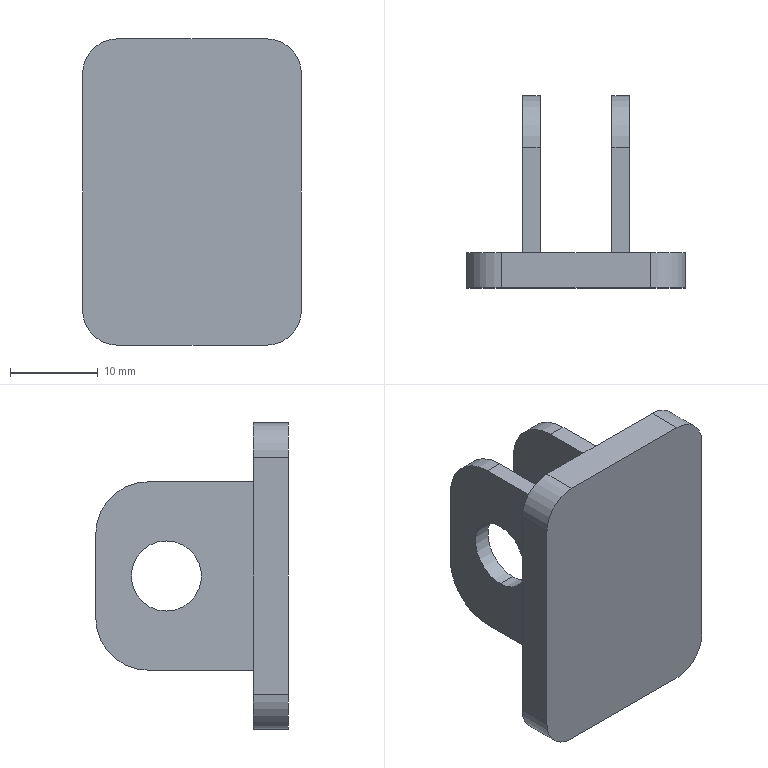Part | SolidWorks | features ICE 2, CosmeticWeldCutList 1, Extrusion 1, Fillet 1 | 1 solid | 28 faces | box 25 x 22 x 35 mm | volume 4732 mm3 | plane 16 | cylinder 12 | commonest cylinder face diameters 8 x8 12 x4
STEP:
#1=CARTESIAN_POINT('',(4.1,13.939,4.));
#2=VERTEX_POINT('',#1);
#3=CARTESIAN_POINT('',(4.1,13.939,-4.));
#4=VERTEX_POINT('',#3);
#5=CARTESIAN_POINT('',(4.1,13.939,0.));
#6=DIRECTION('',(1.,0.,0.));
#7=DIRECTION('',(0.,0.,-1.));
#8=AXIS2_PLACEMENT_3D('',#5,#6,#7);
#9=CIRCLE('',#8,4.);
#10=EDGE_CURVE('',#2,#4,#9,.T.);
#11=ORIENTED_EDGE('',*,*,#10,.F.);
#12=CARTESIAN_POINT('',(6.1,13.939,4.));
#13=VERTEX_POINT('',#12);
#14=CARTESIAN_POINT('',(-12.5,13.939,4.));
#15=DIRECTION('',(1.,0.,0.));
#16=VECTOR('',#15,1000.);
#17=LINE('',#14,#16);
#18=EDGE_CURVE('',#2,#13,#17,.T.);
#19=ORIENTED_EDGE('',*,*,#18,.T.);
#20=CARTESIAN_POINT('',(6.1,13.939,-4.));
#21=VERTEX_POINT('',#20);
#22=CARTESIAN_POINT('',(6.1,13.939,0.));
#23=DIRECTION('',(1.,0.,0.));
#24=DIRECTION('',(0.,0.,-1.));
#25=AXIS2_PLACEMENT_3D('',#22,#23,#24);
#26=CIRCLE('',#25,4.);
#27=EDGE_CURVE('',#13,#21,#26,.T.);
#28=ORIENTED_EDGE('',*,*,#27,.T.);
#29=CARTESIAN_POINT('',(-12.5,13.939,-4.));
#30=DIRECTION('',(1.,0.,0.));
#31=VECTOR('',#30,1000.);
#32=LINE('',#29,#31);
#33=EDGE_CURVE('',#4,#21,#32,.T.);
#34=ORIENTED_EDGE('',*,*,#33,.F.);
#35=EDGE_LOOP('',(#11,#19,#28,#34));
#36=FACE_OUTER_BOUND('',#35,.T.);
#37=CARTESIAN_POINT('',(-12.5,13.939,0.));
#38=DIRECTION('',(1.,0.,0.));
#39=DIRECTION('',(0.,0.,-1.));
#40=AXIS2_PLACEMENT_3D('',#37,#38,#39);
#41=CYLINDRICAL_SURFACE('',#40,4.);
#42=ADVANCED_FACE('',(#36),#41,.F.);
#43=CARTESIAN_POINT('',(-6.1,13.939,4.));
#44=VERTEX_POINT('',#43);
#45=CARTESIAN_POINT('',(-6.1,13.939,-4.));
#46=VERTEX_POINT('',#45);
#47=CARTESIAN_POINT('',(-6.1,13.939,0.));
#48=DIRECTION('',(1.,0.,0.));
#49=DIRECTION('',(0.,0.,-1.));
#50=AXIS2_PLACEMENT_3D('',#47,#48,#49);
#51=CIRCLE('',#50,4.);
#52=EDGE_CURVE('',#44,#46,#51,.T.);
#53=ORIENTED_EDGE('',*,*,#52,.F.);
#54=CARTESIAN_POINT('',(-4.1,13.939,4.));
#55=VERTEX_POINT('',#54);
#56=CARTESIAN_POINT('',(-12.5,13.939,4.));
#57=DIRECTION('',(1.,0.,0.));
#58=VECTOR('',#57,1000.);
#59=LINE('',#56,#58);
#60=EDGE_CURVE('',#44,#55,#59,.T.);
#61=ORIENTED_EDGE('',*,*,#60,.T.);
#62=CARTESIAN_POINT('',(-4.1,13.939,-4.));
#63=VERTEX_POINT('',#62);
#64=CARTESIAN_POINT('',(-4.1,13.939,0.));
#65=DIRECTION('',(-1.,0.,0.));
#66=DIRECTION('',(0.,0.,1.));
#67=AXIS2_PLACEMENT_3D('',#64,#65,#66);
#68=CIRCLE('',#67,4.);
#69=EDGE_CURVE('',#63,#55,#68,.T.);
#70=ORIENTED_EDGE('',*,*,#69,.F.);
#71=CARTESIAN_POINT('',(-12.5,13.939,-4.));
#72=DIRECTION('',(1.,0.,0.));
#73=VECTOR('',#72,1000.);
#74=LINE('',#71,#73);
#75=EDGE_CURVE('',#46,#63,#74,.T.);
#76=ORIENTED_EDGE('',*,*,#75,.F.);
#77=EDGE_LOOP('',(#53,#61,#70,#76));
#78=FACE_OUTER_BOUND('',#77,.T.);
#79=CARTESIAN_POINT('',(-12.5,13.939,0.));
#80=DIRECTION('',(1.,0.,0.));
#81=DIRECTION('',(0.,0.,-1.));
#82=AXIS2_PLACEMENT_3D('',#79,#80,#81);
#83=CYLINDRICAL_SURFACE('',#82,4.);
#84=ADVANCED_FACE('',(#78),#83,.F.);
#85=CARTESIAN_POINT('',(8.5,4.,17.5));
#86=VERTEX_POINT('',#85);
#87=CARTESIAN_POINT('',(12.5,4.,13.5));
#88=VERTEX_POINT('',#87);
#89=CARTESIAN_POINT('',(8.5,4.,13.5));
#90=DIRECTION('',(0.,1.,0.));
#91=DIRECTION('',(0.,0.,1.));
#92=AXIS2_PLACEMENT_3D('',#89,#90,#91);
#93=CIRCLE('',#92,4.);
#94=EDGE_CURVE('',#86,#88,#93,.T.);
#95=ORIENTED_EDGE('',*,*,#94,.T.);
#96=CARTESIAN_POINT('',(12.5,4.,-13.5));
#97=VERTEX_POINT('',#96);
#98=CARTESIAN_POINT('',(12.5,4.,13.5));
#99=DIRECTION('',(0.,0.,-1.));
#100=VECTOR('',#99,1000.);
#101=LINE('',#98,#100);
#102=EDGE_CURVE('',#88,#97,#101,.T.);
#103=ORIENTED_EDGE('',*,*,#102,.T.);
#104=CARTESIAN_POINT('',(8.5,4.,-17.5));
#105=VERTEX_POINT('',#104);
#106=CARTESIAN_POINT('',(8.5,4.,-13.5));
#107=DIRECTION('',(0.,1.,0.));
#108=DIRECTION('',(0.,0.,-1.));
#109=AXIS2_PLACEMENT_3D('',#106,#107,#108);
#110=CIRCLE('',#109,4.);
#111=EDGE_CURVE('',#97,#105,#110,.T.);
#112=ORIENTED_EDGE('',*,*,#111,.T.);
#113=CARTESIAN_POINT('',(-8.5,4.,-17.5));
#114=VERTEX_POINT('',#113);
#115=CARTESIAN_POINT('',(-8.5,4.,-17.5));
#116=DIRECTION('',(-1.,0.,0.));
#117=VECTOR('',#116,1000.);
#118=LINE('',#115,#117);
#119=EDGE_CURVE('',#105,#114,#118,.T.);
#120=ORIENTED_EDGE('',*,*,#119,.T.);
#121=CARTESIAN_POINT('',(-12.5,4.,-13.5));
#122=VERTEX_POINT('',#121);
#123=CARTESIAN_POINT('',(-8.5,4.,-13.5));
#124=DIRECTION('',(0.,1.,0.));
#125=DIRECTION('',(0.,0.,-1.));
#126=AXIS2_PLACEMENT_3D('',#123,#124,#125);
#127=CIRCLE('',#126,4.);
#128=EDGE_CURVE('',#114,#122,#127,.T.);
#129=ORIENTED_EDGE('',*,*,#128,.T.);
#130=CARTESIAN_POINT('',(-12.5,4.,13.5));
#131=VERTEX_POINT('',#130);
#132=CARTESIAN_POINT('',(-12.5,4.,13.5));
#133=DIRECTION('',(0.,0.,1.));
#134=VECTOR('',#133,1000.);
#135=LINE('',#132,#134);
#136=EDGE_CURVE('',#122,#131,#135,.T.);
#137=ORIENTED_EDGE('',*,*,#136,.T.);
#138=CARTESIAN_POINT('',(-8.5,4.,17.5));
#139=VERTEX_POINT('',#138);
#140=CARTESIAN_POINT('',(-8.5,4.,13.5));
#141=DIRECTION('',(0.,1.,0.));
#142=DIRECTION('',(0.,0.,-1.));
#143=AXIS2_PLACEMENT_3D('',#140,#141,#142);
#144=CIRCLE('',#143,4.);
#145=EDGE_CURVE('',#131,#139,#144,.T.);
#146=ORIENTED_EDGE('',*,*,#145,.T.);
#147=CARTESIAN_POINT('',(-8.5,4.,17.5));
#148=DIRECTION('',(1.,0.,0.));
#149=VECTOR('',#148,1000.);
#150=LINE('',#147,#149);
#151=EDGE_CURVE('',#139,#86,#150,.T.);
#152=ORIENTED_EDGE('',*,*,#151,.T.);
#153=EDGE_LOOP('',(#95,#103,#112,#120,#129,#137,#146,#152));
#154=FACE_OUTER_BOUND('',#153,.T.);
#155=CARTESIAN_POINT('',(6.1,4.,-10.761));
#156=VERTEX_POINT('',#155);
#157=CARTESIAN_POINT('',(4.1,4.,-10.761));
#158=VERTEX_POINT('',#157);
#159=CARTESIAN_POINT('',(4.1,4.,-10.761));
#160=DIRECTION('',(-1.,0.,0.));
#161=VECTOR('',#160,1000.);
#162=LINE('',#159,#161);
#163=EDGE_CURVE('',#156,#158,#162,.T.);
#164=ORIENTED_EDGE('',*,*,#163,.F.);
#165=CARTESIAN_POINT('',(6.1,4.,10.761));
#166=VERTEX_POINT('',#165);
#167=CARTESIAN_POINT('',(6.1,4.,-10.761));
#168=DIRECTION('',(0.,0.,-1.));
#169=VECTOR('',#168,1000.);
#170=LINE('',#167,#169);
#171=EDGE_CURVE('',#166,#156,#170,.T.);
#172=ORIENTED_EDGE('',*,*,#171,.F.);
#173=CARTESIAN_POINT('',(4.1,4.,10.761));
#174=VERTEX_POINT('',#173);
#175=CARTESIAN_POINT('',(4.1,4.,10.761));
#176=DIRECTION('',(1.,0.,0.));
#177=VECTOR('',#176,1000.);
#178=LINE('',#175,#177);
#179=EDGE_CURVE('',#174,#166,#178,.T.);
#180=ORIENTED_EDGE('',*,*,#179,.F.);
#181=CARTESIAN_POINT('',(4.1,4.,-10.761));
#182=DIRECTION('',(0.,0.,1.));
#183=VECTOR('',#182,1000.);
#184=LINE('',#181,#183);
#185=EDGE_CURVE('',#158,#174,#184,.T.);
#186=ORIENTED_EDGE('',*,*,#185,.F.);
#187=EDGE_LOOP('',(#164,#172,#180,#186));
#188=FACE_BOUND('',#187,.T.);
#189=CARTESIAN_POINT('',(-6.1,4.,-10.761));
#190=VERTEX_POINT('',#189);
#191=CARTESIAN_POINT('',(-6.1,4.,10.761));
#192=VERTEX_POINT('',#191);
#193=CARTESIAN_POINT('',(-6.1,4.,-10.761));
#194=DIRECTION('',(0.,0.,1.));
#195=VECTOR('',#194,1000.);
#196=LINE('',#193,#195);
#197=EDGE_CURVE('',#190,#192,#196,.T.);
#198=ORIENTED_EDGE('',*,*,#197,.F.);
#199=CARTESIAN_POINT('',(-4.1,4.,-10.761));
#200=VERTEX_POINT('',#199);
#201=CARTESIAN_POINT('',(-4.1,4.,-10.761));
#202=DIRECTION('',(-1.,0.,0.));
#203=VECTOR('',#202,1000.);
#204=LINE('',#201,#203);
#205=EDGE_CURVE('',#200,#190,#204,.T.);
#206=ORIENTED_EDGE('',*,*,#205,.F.);
#207=CARTESIAN_POINT('',(-4.1,4.,10.761));
#208=VERTEX_POINT('',#207);
#209=CARTESIAN_POINT('',(-4.1,4.,-10.761));
#210=DIRECTION('',(0.,0.,-1.));
#211=VECTOR('',#210,1000.);
#212=LINE('',#209,#211);
#213=EDGE_CURVE('',#208,#200,#212,.T.);
#214=ORIENTED_EDGE('',*,*,#213,.F.);
#215=CARTESIAN_POINT('',(-4.1,4.,10.761));
#216=DIRECTION('',(1.,0.,0.));
#217=VECTOR('',#216,1000.);
#218=LINE('',#215,#217);
#219=EDGE_CURVE('',#192,#208,#218,.T.);
#220=ORIENTED_EDGE('',*,*,#219,.F.);
#221=EDGE_LOOP('',(#198,#206,#214,#220));
#222=FACE_BOUND('',#221,.T.);
#223=CARTESIAN_POINT('',(8.5,4.,13.5));
#224=DIRECTION('',(0.,1.,0.));
#225=DIRECTION('',(0.,0.,1.));
#226=AXIS2_PLACEMENT_3D('',#223,#224,#225);
#227=PLANE('',#226);
#228=ADVANCED_FACE('',(#154,#188,#222),#227,.T.);
#229=CARTESIAN_POINT('',(8.5,0.,17.5));
#230=VERTEX_POINT('',#229);
#231=CARTESIAN_POINT('',(12.5,0.,13.5));
#232=VERTEX_POINT('',#231);
#233=CARTESIAN_POINT('',(8.5,0.,13.5));
#234=DIRECTION('',(0.,1.,0.));
#235=DIRECTION('',(0.,0.,1.));
#236=AXIS2_PLACEMENT_3D('',#233,#234,#235);
#237=CIRCLE('',#236,4.);
#238=EDGE_CURVE('',#230,#232,#237,.T.);
#239=ORIENTED_EDGE('',*,*,#238,.T.);
#240=CARTESIAN_POINT('',(12.5,4.,13.5));
#241=DIRECTION('',(0.,-1.,0.));
#242=VECTOR('',#241,1000.);
#243=LINE('',#240,#242);
#244=EDGE_CURVE('',#88,#232,#243,.T.);
#245=ORIENTED_EDGE('',*,*,#244,.F.);
#246=ORIENTED_EDGE('',*,*,#94,.F.);
#247=CARTESIAN_POINT('',(8.5,4.,17.5));
#248=DIRECTION('',(0.,-1.,0.));
#249=VECTOR('',#248,1000.);
#250=LINE('',#247,#249);
#251=EDGE_CURVE('',#86,#230,#250,.T.);
#252=ORIENTED_EDGE('',*,*,#251,.T.);
#253=EDGE_LOOP('',(#239,#245,#246,#252));
#254=FACE_OUTER_BOUND('',#253,.T.);
#255=CARTESIAN_POINT('',(8.5,4.,13.5));
#256=DIRECTION('',(0.,-1.,0.));
#257=DIRECTION('',(0.,0.,-1.));
#258=AXIS2_PLACEMENT_3D('',#255,#256,#257);
#259=CYLINDRICAL_SURFACE('',#258,4.);
#260=ADVANCED_FACE('',(#254),#259,.T.);
#261=CARTESIAN_POINT('',(12.5,0.,-13.5));
#262=VERTEX_POINT('',#261);
#263=CARTESIAN_POINT('',(12.5,0.,13.5));
#264=DIRECTION('',(0.,0.,-1.));
#265=VECTOR('',#264,1000.);
#266=LINE('',#263,#265);
#267=EDGE_CURVE('',#232,#262,#266,.T.);
#268=ORIENTED_EDGE('',*,*,#267,.T.);
#269=CARTESIAN_POINT('',(12.5,4.,-13.5));
#270=DIRECTION('',(0.,-1.,0.));
#271=VECTOR('',#270,1000.);
#272=LINE('',#269,#271);
#273=EDGE_CURVE('',#97,#262,#272,.T.);
#274=ORIENTED_EDGE('',*,*,#273,.F.);
#275=ORIENTED_EDGE('',*,*,#102,.F.);
#276=ORIENTED_EDGE('',*,*,#244,.T.);
#277=EDGE_LOOP('',(#268,#274,#275,#276));
#278=FACE_OUTER_BOUND('',#277,.T.);
#279=CARTESIAN_POINT('',(12.5,4.,13.5));
#280=DIRECTION('',(-1.,0.,0.));
#281=DIRECTION('',(0.,0.,1.));
#282=AXIS2_PLACEMENT_3D('',#279,#280,#281);
#283=PLANE('',#282);
#284=ADVANCED_FACE('',(#278),#283,.F.);
#285=CARTESIAN_POINT('',(8.5,0.,-17.5));
#286=VERTEX_POINT('',#285);
#287=CARTESIAN_POINT('',(8.5,0.,-13.5));
#288=DIRECTION('',(0.,1.,0.));
#289=DIRECTION('',(0.,0.,-1.));
#290=AXIS2_PLACEMENT_3D('',#287,#288,#289);
#291=CIRCLE('',#290,4.);
#292=EDGE_CURVE('',#262,#286,#291,.T.);
#293=ORIENTED_EDGE('',*,*,#292,.T.);
#294=CARTESIAN_POINT('',(8.5,4.,-17.5));
#295=DIRECTION('',(0.,-1.,0.));
#296=VECTOR('',#295,1000.);
#297=LINE('',#294,#296);
#298=EDGE_CURVE('',#105,#286,#297,.T.);
#299=ORIENTED_EDGE('',*,*,#298,.F.);
#300=ORIENTED_EDGE('',*,*,#111,.F.);
#301=ORIENTED_EDGE('',*,*,#273,.T.);
#302=EDGE_LOOP('',(#293,#299,#300,#301));
#303=FACE_OUTER_BOUND('',#302,.T.);
#304=CARTESIAN_POINT('',(8.5,4.,-13.5));
#305=DIRECTION('',(0.,-1.,0.));
#306=DIRECTION('',(0.,0.,-1.));
#307=AXIS2_PLACEMENT_3D('',#304,#305,#306);
#308=CYLINDRICAL_SURFACE('',#307,4.);
#309=ADVANCED_FACE('',(#303),#308,.T.);
#310=CARTESIAN_POINT('',(-8.5,0.,-17.5));
#311=VERTEX_POINT('',#310);
#312=CARTESIAN_POINT('',(-8.5,0.,-17.5));
#313=DIRECTION('',(-1.,0.,0.));
#314=VECTOR('',#313,1000.);
#315=LINE('',#312,#314);
#316=EDGE_CURVE('',#286,#311,#315,.T.);
#317=ORIENTED_EDGE('',*,*,#316,.T.);
#318=CARTESIAN_POINT('',(-8.5,4.,-17.5));
#319=DIRECTION('',(0.,-1.,0.));
#320=VECTOR('',#319,1000.);
#321=LINE('',#318,#320);
#322=EDGE_CURVE('',#114,#311,#321,.T.);
#323=ORIENTED_EDGE('',*,*,#322,.F.);
#324=ORIENTED_EDGE('',*,*,#119,.F.);
#325=ORIENTED_EDGE('',*,*,#298,.T.);
#326=EDGE_LOOP('',(#317,#323,#324,#325));
#327=FACE_OUTER_BOUND('',#326,.T.);
#328=CARTESIAN_POINT('',(-8.5,4.,-17.5));
#329=DIRECTION('',(0.,0.,1.));
#330=DIRECTION('',(1.,0.,0.));
#331=AXIS2_PLACEMENT_3D('',#328,#329,#330);
#332=PLANE('',#331);
#333=ADVANCED_FACE('',(#327),#332,.F.);
#334=CARTESIAN_POINT('',(-12.5,0.,-13.5));
#335=VERTEX_POINT('',#334);
#336=CARTESIAN_POINT('',(-8.5,0.,-13.5));
#337=DIRECTION('',(0.,1.,0.));
#338=DIRECTION('',(0.,0.,-1.));
#339=AXIS2_PLACEMENT_3D('',#336,#337,#338);
#340=CIRCLE('',#339,4.);
#341=EDGE_CURVE('',#311,#335,#340,.T.);
#342=ORIENTED_EDGE('',*,*,#341,.T.);
#343=CARTESIAN_POINT('',(-12.5,4.,-13.5));
#344=DIRECTION('',(0.,-1.,0.));
#345=VECTOR('',#344,1000.);
#346=LINE('',#343,#345);
#347=EDGE_CURVE('',#122,#335,#346,.T.);
#348=ORIENTED_EDGE('',*,*,#347,.F.);
#349=ORIENTED_EDGE('',*,*,#128,.F.);
#350=ORIENTED_EDGE('',*,*,#322,.T.);
#351=EDGE_LOOP('',(#342,#348,#349,#350));
#352=FACE_OUTER_BOUND('',#351,.T.);
#353=CARTESIAN_POINT('',(-8.5,4.,-13.5));
#354=DIRECTION('',(0.,-1.,0.));
#355=DIRECTION('',(0.,0.,-1.));
#356=AXIS2_PLACEMENT_3D('',#353,#354,#355);
#357=CYLINDRICAL_SURFACE('',#356,4.);
#358=ADVANCED_FACE('',(#352),#357,.T.);
#359=CARTESIAN_POINT('',(-12.5,0.,13.5));
#360=VERTEX_POINT('',#359);
#361=CARTESIAN_POINT('',(-12.5,0.,13.5));
#362=DIRECTION('',(0.,0.,1.));
#363=VECTOR('',#362,1000.);
#364=LINE('',#361,#363);
#365=EDGE_CURVE('',#335,#360,#364,.T.);
#366=ORIENTED_EDGE('',*,*,#365,.T.);
#367=CARTESIAN_POINT('',(-12.5,4.,13.5));
#368=DIRECTION('',(0.,-1.,0.));
#369=VECTOR('',#368,1000.);
#370=LINE('',#367,#369);
#371=EDGE_CURVE('',#131,#360,#370,.T.);
#372=ORIENTED_EDGE('',*,*,#371,.F.);
#373=ORIENTED_EDGE('',*,*,#136,.F.);
#374=ORIENTED_EDGE('',*,*,#347,.T.);
#375=EDGE_LOOP('',(#366,#372,#373,#374));
#376=FACE_OUTER_BOUND('',#375,.T.);
#377=CARTESIAN_POINT('',(-12.5,4.,13.5));
#378=DIRECTION('',(1.,0.,0.));
#379=DIRECTION('',(0.,0.,-1.));
#380=AXIS2_PLACEMENT_3D('',#377,#378,#379);
#381=PLANE('',#380);
#382=ADVANCED_FACE('',(#376),#381,.F.);
#383=CARTESIAN_POINT('',(-8.5,0.,17.5));
#384=VERTEX_POINT('',#383);
#385=CARTESIAN_POINT('',(-8.5,0.,13.5));
#386=DIRECTION('',(0.,1.,0.));
#387=DIRECTION('',(0.,0.,-1.));
#388=AXIS2_PLACEMENT_3D('',#385,#386,#387);
#389=CIRCLE('',#388,4.);
#390=EDGE_CURVE('',#360,#384,#389,.T.);
#391=ORIENTED_EDGE('',*,*,#390,.T.);
#392=CARTESIAN_POINT('',(-8.5,4.,17.5));
#393=DIRECTION('',(0.,-1.,0.));
#394=VECTOR('',#393,1000.);
#395=LINE('',#392,#394);
#396=EDGE_CURVE('',#139,#384,#395,.T.);
#397=ORIENTED_EDGE('',*,*,#396,.F.);
#398=ORIENTED_EDGE('',*,*,#145,.F.);
#399=ORIENTED_EDGE('',*,*,#371,.T.);
#400=EDGE_LOOP('',(#391,#397,#398,#399));
#401=FACE_OUTER_BOUND('',#400,.T.);
#402=CARTESIAN_POINT('',(-8.5,4.,13.5));
#403=DIRECTION('',(0.,-1.,0.));
#404=DIRECTION('',(0.,0.,-1.));
#405=AXIS2_PLACEMENT_3D('',#402,#403,#404);
#406=CYLINDRICAL_SURFACE('',#405,4.);
#407=ADVANCED_FACE('',(#401),#406,.T.);
#408=CARTESIAN_POINT('',(-8.5,0.,17.5));
#409=DIRECTION('',(1.,0.,0.));
#410=VECTOR('',#409,1000.);
#411=LINE('',#408,#410);
#412=EDGE_CURVE('',#384,#230,#411,.T.);
#413=ORIENTED_EDGE('',*,*,#412,.T.);
#414=ORIENTED_EDGE('',*,*,#251,.F.);
#415=ORIENTED_EDGE('',*,*,#151,.F.);
#416=ORIENTED_EDGE('',*,*,#396,.T.);
#417=EDGE_LOOP('',(#413,#414,#415,#416));
#418=FACE_OUTER_BOUND('',#417,.T.);
#419=CARTESIAN_POINT('',(-8.5,4.,17.5));
#420=DIRECTION('',(0.,0.,-1.));
#421=DIRECTION('',(-1.,0.,0.));
#422=AXIS2_PLACEMENT_3D('',#419,#420,#421);
#423=PLANE('',#422);
#424=ADVANCED_FACE('',(#418),#423,.F.);
#425=ORIENTED_EDGE('',*,*,#238,.F.);
#426=ORIENTED_EDGE('',*,*,#412,.F.);
#427=ORIENTED_EDGE('',*,*,#390,.F.);
#428=ORIENTED_EDGE('',*,*,#365,.F.);
#429=ORIENTED_EDGE('',*,*,#341,.F.);
#430=ORIENTED_EDGE('',*,*,#316,.F.);
#431=ORIENTED_EDGE('',*,*,#292,.F.);
#432=ORIENTED_EDGE('',*,*,#267,.F.);
#433=EDGE_LOOP('',(#425,#426,#427,#428,#429,#430,#431,#432));
#434=FACE_OUTER_BOUND('',#433,.T.);
#435=CARTESIAN_POINT('',(8.5,0.,13.5));
#436=DIRECTION('',(0.,1.,0.));
#437=DIRECTION('',(0.,0.,1.));
#438=AXIS2_PLACEMENT_3D('',#435,#436,#437);
#439=PLANE('',#438);
#440=ADVANCED_FACE('',(#434),#439,.F.);
#441=CARTESIAN_POINT('',(6.1,13.939,0.));
#442=DIRECTION('',(1.,0.,0.));
#443=DIRECTION('',(0.,0.,-1.));
#444=AXIS2_PLACEMENT_3D('',#441,#442,#443);
#445=CIRCLE('',#444,4.);
#446=EDGE_CURVE('',#21,#13,#445,.T.);
#447=ORIENTED_EDGE('',*,*,#446,.F.);
#448=ORIENTED_EDGE('',*,*,#27,.F.);
#449=EDGE_LOOP('',(#447,#448));
#450=FACE_BOUND('',#449,.T.);
#451=CARTESIAN_POINT('',(6.1,16.,-10.761));
#452=VERTEX_POINT('',#451);
#453=CARTESIAN_POINT('',(6.1,22.,-10.761));
#454=DIRECTION('',(0.,-1.,0.));
#455=VECTOR('',#454,1000.);
#456=LINE('',#453,#455);
#457=EDGE_CURVE('',#452,#156,#456,.T.);
#458=ORIENTED_EDGE('',*,*,#457,.F.);
#459=CARTESIAN_POINT('',(6.1,22.,-4.761));
#460=VERTEX_POINT('',#459);
#461=CARTESIAN_POINT('',(6.1,16.,-4.761));
#462=DIRECTION('',(1.,0.,0.));
#463=DIRECTION('',(0.,0.,1.));
#464=AXIS2_PLACEMENT_3D('',#461,#462,#463);
#465=CIRCLE('',#464,6.);
#466=EDGE_CURVE('',#452,#460,#465,.T.);
#467=ORIENTED_EDGE('',*,*,#466,.T.);
#468=CARTESIAN_POINT('',(6.1,22.,4.761));
#469=VERTEX_POINT('',#468);
#470=CARTESIAN_POINT('',(6.1,22.,-10.761));
#471=DIRECTION('',(0.,0.,-1.));
#472=VECTOR('',#471,1000.);
#473=LINE('',#470,#472);
#474=EDGE_CURVE('',#469,#460,#473,.T.);
#475=ORIENTED_EDGE('',*,*,#474,.F.);
#476=CARTESIAN_POINT('',(6.1,16.,10.761));
#477=VERTEX_POINT('',#476);
#478=CARTESIAN_POINT('',(6.1,16.,4.761));
#479=DIRECTION('',(1.,0.,0.));
#480=DIRECTION('',(0.,0.,1.));
#481=AXIS2_PLACEMENT_3D('',#478,#479,#480);
#482=CIRCLE('',#481,6.);
#483=EDGE_CURVE('',#469,#477,#482,.T.);
#484=ORIENTED_EDGE('',*,*,#483,.T.);
#485=CARTESIAN_POINT('',(6.1,22.,10.761));
#486=DIRECTION('',(0.,-1.,0.));
#487=VECTOR('',#486,1000.);
#488=LINE('',#485,#487);
#489=EDGE_CURVE('',#477,#166,#488,.T.);
#490=ORIENTED_EDGE('',*,*,#489,.T.);
#491=ORIENTED_EDGE('',*,*,#171,.T.);
#492=EDGE_LOOP('',(#458,#467,#475,#484,#490,#491));
#493=FACE_OUTER_BOUND('',#492,.T.);
#494=CARTESIAN_POINT('',(6.1,22.,-10.761));
#495=DIRECTION('',(-1.,0.,0.));
#496=DIRECTION('',(0.,0.,1.));
#497=AXIS2_PLACEMENT_3D('',#494,#495,#496);
#498=PLANE('',#497);
#499=ADVANCED_FACE('',(#450,#493),#498,.F.);
#500=CARTESIAN_POINT('',(4.1,16.,-10.761));
#501=VERTEX_POINT('',#500);
#502=CARTESIAN_POINT('',(4.1,22.,-10.761));
#503=DIRECTION('',(0.,-1.,0.));
#504=VECTOR('',#503,1000.);
#505=LINE('',#502,#504);
#506=EDGE_CURVE('',#501,#158,#505,.T.);
#507=ORIENTED_EDGE('',*,*,#506,.F.);
#508=CARTESIAN_POINT('',(6.1,16.,-10.761));
#509=DIRECTION('',(1.,0.,0.));
#510=VECTOR('',#509,1000.);
#511=LINE('',#508,#510);
#512=EDGE_CURVE('',#501,#452,#511,.T.);
#513=ORIENTED_EDGE('',*,*,#512,.T.);
#514=ORIENTED_EDGE('',*,*,#457,.T.);
#515=ORIENTED_EDGE('',*,*,#163,.T.);
#516=EDGE_LOOP('',(#507,#513,#514,#515));
#517=FACE_OUTER_BOUND('',#516,.T.);
#518=CARTESIAN_POINT('',(4.1,22.,-10.761));
#519=DIRECTION('',(0.,0.,1.));
#520=DIRECTION('',(1.,0.,0.));
#521=AXIS2_PLACEMENT_3D('',#518,#519,#520);
#522=PLANE('',#521);
#523=ADVANCED_FACE('',(#517),#522,.F.);
#524=CARTESIAN_POINT('',(4.1,13.939,0.));
#525=DIRECTION('',(1.,0.,0.));
#526=DIRECTION('',(0.,0.,-1.));
#527=AXIS2_PLACEMENT_3D('',#524,#525,#526);
#528=CIRCLE('',#527,4.);
#529=EDGE_CURVE('',#4,#2,#528,.T.);
#530=ORIENTED_EDGE('',*,*,#529,.T.);
#531=ORIENTED_EDGE('',*,*,#10,.T.);
#532=EDGE_LOOP('',(#530,#531));
#533=FACE_BOUND('',#532,.T.);
#534=CARTESIAN_POINT('',(4.1,22.,-4.761));
#535=VERTEX_POINT('',#534);
#536=CARTESIAN_POINT('',(4.1,22.,4.761));
#537=VERTEX_POINT('',#536);
#538=CARTESIAN_POINT('',(4.1,22.,-10.761));
#539=DIRECTION('',(0.,0.,1.));
#540=VECTOR('',#539,1000.);
#541=LINE('',#538,#540);
#542=EDGE_CURVE('',#535,#537,#541,.T.);
#543=ORIENTED_EDGE('',*,*,#542,.F.);
#544=CARTESIAN_POINT('',(4.1,16.,-4.761));
#545=DIRECTION('',(-1.,0.,0.));
#546=DIRECTION('',(0.,0.,-1.));
#547=AXIS2_PLACEMENT_3D('',#544,#545,#546);
#548=CIRCLE('',#547,6.);
#549=EDGE_CURVE('',#535,#501,#548,.T.);
#550=ORIENTED_EDGE('',*,*,#549,.T.);
#551=ORIENTED_EDGE('',*,*,#506,.T.);
#552=ORIENTED_EDGE('',*,*,#185,.T.);
#553=CARTESIAN_POINT('',(4.1,16.,10.761));
#554=VERTEX_POINT('',#553);
#555=CARTESIAN_POINT('',(4.1,22.,10.761));
#556=DIRECTION('',(0.,-1.,0.));
#557=VECTOR('',#556,1000.);
#558=LINE('',#555,#557);
#559=EDGE_CURVE('',#554,#174,#558,.T.);
#560=ORIENTED_EDGE('',*,*,#559,.F.);
#561=CARTESIAN_POINT('',(4.1,16.,4.761));
#562=DIRECTION('',(-1.,0.,0.));
#563=DIRECTION('',(0.,0.,-1.));
#564=AXIS2_PLACEMENT_3D('',#561,#562,#563);
#565=CIRCLE('',#564,6.);
#566=EDGE_CURVE('',#554,#537,#565,.T.);
#567=ORIENTED_EDGE('',*,*,#566,.T.);
#568=EDGE_LOOP('',(#543,#550,#551,#552,#560,#567));
#569=FACE_OUTER_BOUND('',#568,.T.);
#570=CARTESIAN_POINT('',(4.1,22.,-10.761));
#571=DIRECTION('',(1.,0.,0.));
#572=DIRECTION('',(0.,0.,-1.));
#573=AXIS2_PLACEMENT_3D('',#570,#571,#572);
#574=PLANE('',#573);
#575=ADVANCED_FACE('',(#533,#569),#574,.F.);
#576=ORIENTED_EDGE('',*,*,#489,.F.);
#577=CARTESIAN_POINT('',(4.1,16.,10.761));
#578=DIRECTION('',(-1.,0.,0.));
#579=VECTOR('',#578,1000.);
#580=LINE('',#577,#579);
#581=EDGE_CURVE('',#477,#554,#580,.T.);
#582=ORIENTED_EDGE('',*,*,#581,.T.);
#583=ORIENTED_EDGE('',*,*,#559,.T.);
#584=ORIENTED_EDGE('',*,*,#179,.T.);
#585=EDGE_LOOP('',(#576,#582,#583,#584));
#586=FACE_OUTER_BOUND('',#585,.T.);
#587=CARTESIAN_POINT('',(4.1,22.,10.761));
#588=DIRECTION('',(0.,0.,-1.));
#589=DIRECTION('',(-1.,0.,0.));
#590=AXIS2_PLACEMENT_3D('',#587,#588,#589);
#591=PLANE('',#590);
#592=ADVANCED_FACE('',(#586),#591,.F.);
#593=ORIENTED_EDGE('',*,*,#474,.T.);
#594=CARTESIAN_POINT('',(4.1,22.,-4.761));
#595=DIRECTION('',(-1.,0.,0.));
#596=VECTOR('',#595,1000.);
#597=LINE('',#594,#596);
#598=EDGE_CURVE('',#460,#535,#597,.T.);
#599=ORIENTED_EDGE('',*,*,#598,.T.);
#600=ORIENTED_EDGE('',*,*,#542,.T.);
#601=CARTESIAN_POINT('',(6.1,22.,4.761));
#602=DIRECTION('',(1.,0.,0.));
#603=VECTOR('',#602,1000.);
#604=LINE('',#601,#603);
#605=EDGE_CURVE('',#537,#469,#604,.T.);
#606=ORIENTED_EDGE('',*,*,#605,.T.);
#607=EDGE_LOOP('',(#593,#599,#600,#606));
#608=FACE_OUTER_BOUND('',#607,.T.);
#609=CARTESIAN_POINT('',(0.,22.,0.));
#610=DIRECTION('',(0.,1.,0.));
#611=DIRECTION('',(0.,0.,1.));
#612=AXIS2_PLACEMENT_3D('',#609,#610,#611);
#613=PLANE('',#612);
#614=ADVANCED_FACE('',(#608),#613,.T.);
#615=CARTESIAN_POINT('',(-6.1,16.,-10.761));
#616=VERTEX_POINT('',#615);
#617=CARTESIAN_POINT('',(-6.1,22.,-10.761));
#618=DIRECTION('',(0.,-1.,0.));
#619=VECTOR('',#618,1000.);
#620=LINE('',#617,#619);
#621=EDGE_CURVE('',#616,#190,#620,.T.);
#622=ORIENTED_EDGE('',*,*,#621,.F.);
#623=CARTESIAN_POINT('',(-4.1,16.,-10.761));
#624=VERTEX_POINT('',#623);
#625=CARTESIAN_POINT('',(-4.1,16.,-10.761));
#626=DIRECTION('',(1.,0.,0.));
#627=VECTOR('',#626,1000.);
#628=LINE('',#625,#627);
#629=EDGE_CURVE('',#616,#624,#628,.T.);
#630=ORIENTED_EDGE('',*,*,#629,.T.);
#631=CARTESIAN_POINT('',(-4.1,22.,-10.761));
#632=DIRECTION('',(0.,-1.,0.));
#633=VECTOR('',#632,1000.);
#634=LINE('',#631,#633);
#635=EDGE_CURVE('',#624,#200,#634,.T.);
#636=ORIENTED_EDGE('',*,*,#635,.T.);
#637=ORIENTED_EDGE('',*,*,#205,.T.);
#638=EDGE_LOOP('',(#622,#630,#636,#637));
#639=FACE_OUTER_BOUND('',#638,.T.);
#640=CARTESIAN_POINT('',(-4.1,22.,-10.761));
#641=DIRECTION('',(0.,0.,1.));
#642=DIRECTION('',(1.,0.,0.));
#643=AXIS2_PLACEMENT_3D('',#640,#641,#642);
#644=PLANE('',#643);
#645=ADVANCED_FACE('',(#639),#644,.F.);
#646=CARTESIAN_POINT('',(-6.1,13.939,0.));
#647=DIRECTION('',(1.,0.,0.));
#648=DIRECTION('',(0.,0.,-1.));
#649=AXIS2_PLACEMENT_3D('',#646,#647,#648);
#650=CIRCLE('',#649,4.);
#651=EDGE_CURVE('',#46,#44,#650,.T.);
#652=ORIENTED_EDGE('',*,*,#651,.T.);
#653=ORIENTED_EDGE('',*,*,#52,.T.);
#654=EDGE_LOOP('',(#652,#653));
#655=FACE_BOUND('',#654,.T.);
#656=CARTESIAN_POINT('',(-6.1,22.,-4.761));
#657=VERTEX_POINT('',#656);
#658=CARTESIAN_POINT('',(-6.1,22.,4.761));
#659=VERTEX_POINT('',#658);
#660=CARTESIAN_POINT('',(-6.1,22.,-10.761));
#661=DIRECTION('',(0.,0.,1.));
#662=VECTOR('',#661,1000.);
#663=LINE('',#660,#662);
#664=EDGE_CURVE('',#657,#659,#663,.T.);
#665=ORIENTED_EDGE('',*,*,#664,.F.);
#666=CARTESIAN_POINT('',(-6.1,16.,-4.761));
#667=DIRECTION('',(-1.,0.,0.));
#668=DIRECTION('',(0.,0.,-1.));
#669=AXIS2_PLACEMENT_3D('',#666,#667,#668);
#670=CIRCLE('',#669,6.);
#671=EDGE_CURVE('',#657,#616,#670,.T.);
#672=ORIENTED_EDGE('',*,*,#671,.T.);
#673=ORIENTED_EDGE('',*,*,#621,.T.);
#674=ORIENTED_EDGE('',*,*,#197,.T.);
#675=CARTESIAN_POINT('',(-6.1,16.,10.761));
#676=VERTEX_POINT('',#675);
#677=CARTESIAN_POINT('',(-6.1,22.,10.761));
#678=DIRECTION('',(0.,-1.,0.));
#679=VECTOR('',#678,1000.);
#680=LINE('',#677,#679);
#681=EDGE_CURVE('',#676,#192,#680,.T.);
#682=ORIENTED_EDGE('',*,*,#681,.F.);
#683=CARTESIAN_POINT('',(-6.1,16.,4.761));
#684=DIRECTION('',(-1.,0.,0.));
#685=DIRECTION('',(0.,0.,-1.));
#686=AXIS2_PLACEMENT_3D('',#683,#684,#685);
#687=CIRCLE('',#686,6.);
#688=EDGE_CURVE('',#676,#659,#687,.T.);
#689=ORIENTED_EDGE('',*,*,#688,.T.);
#690=EDGE_LOOP('',(#665,#672,#673,#674,#682,#689));
#691=FACE_OUTER_BOUND('',#690,.T.);
#692=CARTESIAN_POINT('',(-6.1,22.,-10.761));
#693=DIRECTION('',(1.,0.,0.));
#694=DIRECTION('',(0.,0.,-1.));
#695=AXIS2_PLACEMENT_3D('',#692,#693,#694);
#696=PLANE('',#695);
#697=ADVANCED_FACE('',(#655,#691),#696,.F.);
#698=CARTESIAN_POINT('',(-4.1,16.,10.761));
#699=VERTEX_POINT('',#698);
#700=CARTESIAN_POINT('',(-4.1,22.,10.761));
#701=DIRECTION('',(0.,-1.,0.));
#702=VECTOR('',#701,1000.);
#703=LINE('',#700,#702);
#704=EDGE_CURVE('',#699,#208,#703,.T.);
#705=ORIENTED_EDGE('',*,*,#704,.F.);
#706=CARTESIAN_POINT('',(-6.1,16.,10.761));
#707=DIRECTION('',(-1.,0.,0.));
#708=VECTOR('',#707,1000.);
#709=LINE('',#706,#708);
#710=EDGE_CURVE('',#699,#676,#709,.T.);
#711=ORIENTED_EDGE('',*,*,#710,.T.);
#712=ORIENTED_EDGE('',*,*,#681,.T.);
#713=ORIENTED_EDGE('',*,*,#219,.T.);
#714=EDGE_LOOP('',(#705,#711,#712,#713));
#715=FACE_OUTER_BOUND('',#714,.T.);
#716=CARTESIAN_POINT('',(-4.1,22.,10.761));
#717=DIRECTION('',(0.,0.,-1.));
#718=DIRECTION('',(-1.,0.,0.));
#719=AXIS2_PLACEMENT_3D('',#716,#717,#718);
#720=PLANE('',#719);
#721=ADVANCED_FACE('',(#715),#720,.F.);
#722=ORIENTED_EDGE('',*,*,#69,.T.);
#723=CARTESIAN_POINT('',(-4.1,13.939,0.));
#724=DIRECTION('',(-1.,0.,0.));
#725=DIRECTION('',(0.,0.,1.));
#726=AXIS2_PLACEMENT_3D('',#723,#724,#725);
#727=CIRCLE('',#726,4.);
#728=EDGE_CURVE('',#55,#63,#727,.T.);
#729=ORIENTED_EDGE('',*,*,#728,.T.);
#730=EDGE_LOOP('',(#722,#729));
#731=FACE_BOUND('',#730,.T.);
#732=ORIENTED_EDGE('',*,*,#635,.F.);
#733=CARTESIAN_POINT('',(-4.1,22.,-4.761));
#734=VERTEX_POINT('',#733);
#735=CARTESIAN_POINT('',(-4.1,16.,-4.761));
#736=DIRECTION('',(1.,0.,0.));
#737=DIRECTION('',(0.,0.,1.));
#738=AXIS2_PLACEMENT_3D('',#735,#736,#737);
#739=CIRCLE('',#738,6.);
#740=EDGE_CURVE('',#624,#734,#739,.T.);
#741=ORIENTED_EDGE('',*,*,#740,.T.);
#742=CARTESIAN_POINT('',(-4.1,22.,4.761));
#743=VERTEX_POINT('',#742);
#744=CARTESIAN_POINT('',(-4.1,22.,-10.761));
#745=DIRECTION('',(0.,0.,-1.));
#746=VECTOR('',#745,1000.);
#747=LINE('',#744,#746);
#748=EDGE_CURVE('',#743,#734,#747,.T.);
#749=ORIENTED_EDGE('',*,*,#748,.F.);
#750=CARTESIAN_POINT('',(-4.1,16.,4.761));
#751=DIRECTION('',(1.,0.,0.));
#752=DIRECTION('',(0.,0.,1.));
#753=AXIS2_PLACEMENT_3D('',#750,#751,#752);
#754=CIRCLE('',#753,6.);
#755=EDGE_CURVE('',#743,#699,#754,.T.);
#756=ORIENTED_EDGE('',*,*,#755,.T.);
#757=ORIENTED_EDGE('',*,*,#704,.T.);
#758=ORIENTED_EDGE('',*,*,#213,.T.);
#759=EDGE_LOOP('',(#732,#741,#749,#756,#757,#758));
#760=FACE_OUTER_BOUND('',#759,.T.);
#761=CARTESIAN_POINT('',(-4.1,22.,-10.761));
#762=DIRECTION('',(-1.,0.,0.));
#763=DIRECTION('',(0.,0.,1.));
#764=AXIS2_PLACEMENT_3D('',#761,#762,#763);
#765=PLANE('',#764);
#766=ADVANCED_FACE('',(#731,#760),#765,.F.);
#767=ORIENTED_EDGE('',*,*,#748,.T.);
#768=CARTESIAN_POINT('',(-6.1,22.,-4.761));
#769=DIRECTION('',(-1.,0.,0.));
#770=VECTOR('',#769,1000.);
#771=LINE('',#768,#770);
#772=EDGE_CURVE('',#734,#657,#771,.T.);
#773=ORIENTED_EDGE('',*,*,#772,.T.);
#774=ORIENTED_EDGE('',*,*,#664,.T.);
#775=CARTESIAN_POINT('',(-4.1,22.,4.761));
#776=DIRECTION('',(1.,0.,0.));
#777=VECTOR('',#776,1000.);
#778=LINE('',#775,#777);
#779=EDGE_CURVE('',#659,#743,#778,.T.);
#780=ORIENTED_EDGE('',*,*,#779,.T.);
#781=EDGE_LOOP('',(#767,#773,#774,#780));
#782=FACE_OUTER_BOUND('',#781,.T.);
#783=CARTESIAN_POINT('',(0.,22.,0.));
#784=DIRECTION('',(0.,1.,0.));
#785=DIRECTION('',(0.,0.,1.));
#786=AXIS2_PLACEMENT_3D('',#783,#784,#785);
#787=PLANE('',#786);
#788=ADVANCED_FACE('',(#782),#787,.T.);
#789=ORIENTED_EDGE('',*,*,#740,.F.);
#790=ORIENTED_EDGE('',*,*,#629,.F.);
#791=ORIENTED_EDGE('',*,*,#671,.F.);
#792=ORIENTED_EDGE('',*,*,#772,.F.);
#793=EDGE_LOOP('',(#789,#790,#791,#792));
#794=FACE_OUTER_BOUND('',#793,.T.);
#795=CARTESIAN_POINT('',(0.,16.,-4.761));
#796=DIRECTION('',(1.,0.,0.));
#797=DIRECTION('',(0.,0.,-1.));
#798=AXIS2_PLACEMENT_3D('',#795,#796,#797);
#799=CYLINDRICAL_SURFACE('',#798,6.);
#800=ADVANCED_FACE('',(#794),#799,.T.);
#801=ORIENTED_EDGE('',*,*,#466,.F.);
#802=ORIENTED_EDGE('',*,*,#512,.F.);
#803=ORIENTED_EDGE('',*,*,#549,.F.);
#804=ORIENTED_EDGE('',*,*,#598,.F.);
#805=EDGE_LOOP('',(#801,#802,#803,#804));
#806=FACE_OUTER_BOUND('',#805,.T.);
#807=CARTESIAN_POINT('',(0.,16.,-4.761));
#808=DIRECTION('',(1.,0.,0.));
#809=DIRECTION('',(0.,0.,-1.));
#810=AXIS2_PLACEMENT_3D('',#807,#808,#809);
#811=CYLINDRICAL_SURFACE('',#810,6.);
#812=ADVANCED_FACE('',(#806),#811,.T.);
#813=ORIENTED_EDGE('',*,*,#566,.F.);
#814=ORIENTED_EDGE('',*,*,#581,.F.);
#815=ORIENTED_EDGE('',*,*,#483,.F.);
#816=ORIENTED_EDGE('',*,*,#605,.F.);
#817=EDGE_LOOP('',(#813,#814,#815,#816));
#818=FACE_OUTER_BOUND('',#817,.T.);
#819=CARTESIAN_POINT('',(0.,16.,4.761));
#820=DIRECTION('',(-1.,0.,0.));
#821=DIRECTION('',(0.,0.,1.));
#822=AXIS2_PLACEMENT_3D('',#819,#820,#821);
#823=CYLINDRICAL_SURFACE('',#822,6.);
#824=ADVANCED_FACE('',(#818),#823,.T.);
#825=ORIENTED_EDGE('',*,*,#688,.F.);
#826=ORIENTED_EDGE('',*,*,#710,.F.);
#827=ORIENTED_EDGE('',*,*,#755,.F.);
#828=ORIENTED_EDGE('',*,*,#779,.F.);
#829=EDGE_LOOP('',(#825,#826,#827,#828));
#830=FACE_OUTER_BOUND('',#829,.T.);
#831=CARTESIAN_POINT('',(0.,16.,4.761));
#832=DIRECTION('',(-1.,0.,0.));
#833=DIRECTION('',(0.,0.,1.));
#834=AXIS2_PLACEMENT_3D('',#831,#832,#833);
#835=CYLINDRICAL_SURFACE('',#834,6.);
#836=ADVANCED_FACE('',(#830),#835,.T.);
#837=ORIENTED_EDGE('',*,*,#60,.F.);
#838=ORIENTED_EDGE('',*,*,#651,.F.);
#839=ORIENTED_EDGE('',*,*,#75,.T.);
#840=ORIENTED_EDGE('',*,*,#728,.F.);
#841=EDGE_LOOP('',(#837,#838,#839,#840));
#842=FACE_OUTER_BOUND('',#841,.T.);
#843=CARTESIAN_POINT('',(-12.5,13.939,0.));
#844=DIRECTION('',(1.,0.,0.));
#845=DIRECTION('',(0.,0.,-1.));
#846=AXIS2_PLACEMENT_3D('',#843,#844,#845);
#847=CYLINDRICAL_SURFACE('',#846,4.);
#848=ADVANCED_FACE('',(#842),#847,.F.);
#849=ORIENTED_EDGE('',*,*,#18,.F.);
#850=ORIENTED_EDGE('',*,*,#529,.F.);
#851=ORIENTED_EDGE('',*,*,#33,.T.);
#852=ORIENTED_EDGE('',*,*,#446,.T.);
#853=EDGE_LOOP('',(#849,#850,#851,#852));
#854=FACE_OUTER_BOUND('',#853,.T.);
#855=CARTESIAN_POINT('',(-12.5,13.939,0.));
#856=DIRECTION('',(1.,0.,0.));
#857=DIRECTION('',(0.,0.,-1.));
#858=AXIS2_PLACEMENT_3D('',#855,#856,#857);
#859=CYLINDRICAL_SURFACE('',#858,4.);
#860=ADVANCED_FACE('',(#854),#859,.F.);
#861=CLOSED_SHELL('',(#42,#84,#228,#260,#284,#309,#333,#358,#382,#407,#424,#440,#499,#523,#575,#592,#614,#645,#697,#721,#766,#788,#800,#812,#824,#836,#848,#860));
#862=MANIFOLD_SOLID_BREP('',#861);
#863=CARTESIAN_POINT('',(0.,0.,0.));
#864=DIRECTION('',(0.,0.,1.));
#865=DIRECTION('',(1.,0.,0.));
#866=AXIS2_PLACEMENT_3D('',#863,#864,#865);
#867=(LENGTH_UNIT()NAMED_UNIT(*)SI_UNIT(.MILLI.,.METRE.));
#868=UNCERTAINTY_MEASURE_WITH_UNIT(LENGTH_MEASURE(0.00001),#867,'','');
#869=(NAMED_UNIT(*)PLANE_ANGLE_UNIT()SI_UNIT($,.RADIAN.));
#870=(NAMED_UNIT(*)SI_UNIT($,.STERADIAN.)SOLID_ANGLE_UNIT());
#871=(GEOMETRIC_REPRESENTATION_CONTEXT(3)GLOBAL_UNCERTAINTY_ASSIGNED_CONTEXT((#868))GLOBAL_UNIT_ASSIGNED_CONTEXT((#867,#869,#870))REPRESENTATION_CONTEXT('',''));
#872=ADVANCED_BREP_SHAPE_REPRESENTATION('',(#862,#866),#871);